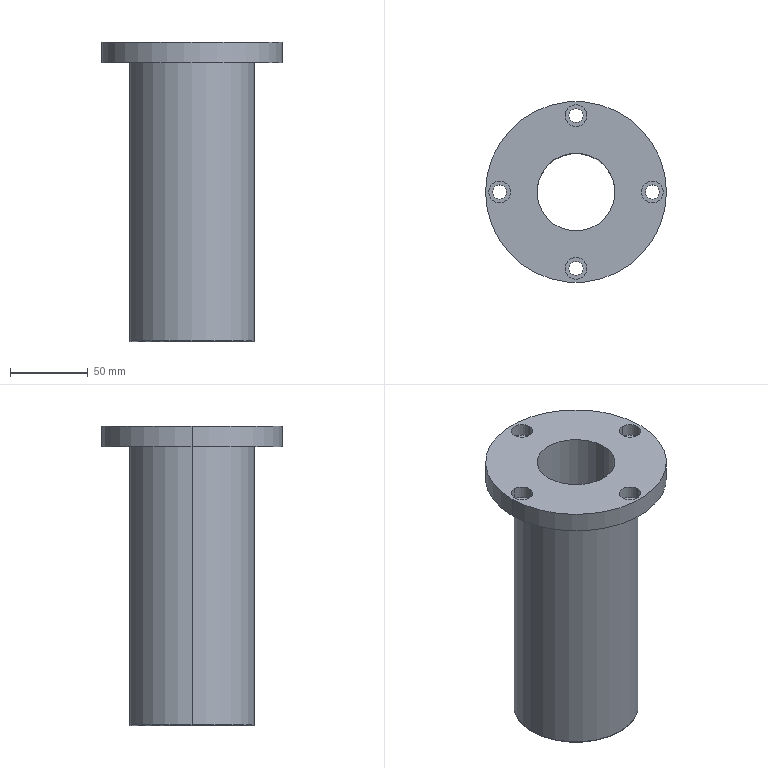Part | SolidWorks | features CirPattern 1, Fillet 1, ICE 1, RevCut 1, Revolution 1 | 1 solid | 31 faces | box 116 x 116 x 192 mm | volume 653901 mm3 | cylinder 22 | plane 7 | torus 2 | commonest cylinder face diameters 9 x8 14 x8 50 x2 80 x2 116 x2
STEP:
#1=CARTESIAN_POINT('',(49.,4.5,0.));
#2=VERTEX_POINT('',#1);
#3=CARTESIAN_POINT('',(49.,-4.5,0.));
#4=VERTEX_POINT('',#3);
#5=CARTESIAN_POINT('',(49.,0.,0.));
#6=DIRECTION('',(0.,0.,1.));
#7=DIRECTION('',(0.,-1.,0.));
#8=AXIS2_PLACEMENT_3D('',#5,#6,#7);
#9=CIRCLE('',#8,4.5);
#10=EDGE_CURVE('',#2,#4,#9,.T.);
#11=ORIENTED_EDGE('',*,*,#10,.F.);
#12=CARTESIAN_POINT('',(49.,4.5,4.9));
#13=VERTEX_POINT('',#12);
#14=CARTESIAN_POINT('',(49.,4.5,0.));
#15=DIRECTION('',(0.,0.,1.));
#16=VECTOR('',#15,1000.);
#17=LINE('',#14,#16);
#18=EDGE_CURVE('',#2,#13,#17,.T.);
#19=ORIENTED_EDGE('',*,*,#18,.T.);
#20=CARTESIAN_POINT('',(49.,-4.5,4.9));
#21=VERTEX_POINT('',#20);
#22=CARTESIAN_POINT('',(49.,0.,4.9));
#23=DIRECTION('',(0.,0.,1.));
#24=DIRECTION('',(0.,-1.,0.));
#25=AXIS2_PLACEMENT_3D('',#22,#23,#24);
#26=CIRCLE('',#25,4.5);
#27=EDGE_CURVE('',#13,#21,#26,.T.);
#28=ORIENTED_EDGE('',*,*,#27,.T.);
#29=CARTESIAN_POINT('',(49.,-4.5,0.));
#30=DIRECTION('',(0.,0.,1.));
#31=VECTOR('',#30,1000.);
#32=LINE('',#29,#31);
#33=EDGE_CURVE('',#4,#21,#32,.T.);
#34=ORIENTED_EDGE('',*,*,#33,.F.);
#35=EDGE_LOOP('',(#11,#19,#28,#34));
#36=FACE_OUTER_BOUND('',#35,.T.);
#37=CARTESIAN_POINT('',(49.,0.,0.));
#38=DIRECTION('',(0.,0.,1.));
#39=DIRECTION('',(0.,-1.,0.));
#40=AXIS2_PLACEMENT_3D('',#37,#38,#39);
#41=CYLINDRICAL_SURFACE('',#40,4.5);
#42=ADVANCED_FACE('',(#36),#41,.F.);
#43=CARTESIAN_POINT('',(49.,7.,4.9));
#44=VERTEX_POINT('',#43);
#45=CARTESIAN_POINT('',(49.,-7.,4.9));
#46=VERTEX_POINT('',#45);
#47=CARTESIAN_POINT('',(49.,0.,4.9));
#48=DIRECTION('',(0.,0.,1.));
#49=DIRECTION('',(0.,-1.,0.));
#50=AXIS2_PLACEMENT_3D('',#47,#48,#49);
#51=CIRCLE('',#50,7.);
#52=EDGE_CURVE('',#44,#46,#51,.T.);
#53=ORIENTED_EDGE('',*,*,#52,.F.);
#54=CARTESIAN_POINT('',(49.,7.,13.));
#55=VERTEX_POINT('',#54);
#56=CARTESIAN_POINT('',(49.,7.,0.));
#57=DIRECTION('',(0.,0.,1.));
#58=VECTOR('',#57,1000.);
#59=LINE('',#56,#58);
#60=EDGE_CURVE('',#44,#55,#59,.T.);
#61=ORIENTED_EDGE('',*,*,#60,.T.);
#62=CARTESIAN_POINT('',(49.,-7.,13.));
#63=VERTEX_POINT('',#62);
#64=CARTESIAN_POINT('',(49.,0.,13.));
#65=DIRECTION('',(0.,0.,1.));
#66=DIRECTION('',(0.,-1.,0.));
#67=AXIS2_PLACEMENT_3D('',#64,#65,#66);
#68=CIRCLE('',#67,7.);
#69=EDGE_CURVE('',#55,#63,#68,.T.);
#70=ORIENTED_EDGE('',*,*,#69,.T.);
#71=CARTESIAN_POINT('',(49.,-7.,0.));
#72=DIRECTION('',(0.,0.,1.));
#73=VECTOR('',#72,1000.);
#74=LINE('',#71,#73);
#75=EDGE_CURVE('',#46,#63,#74,.T.);
#76=ORIENTED_EDGE('',*,*,#75,.F.);
#77=EDGE_LOOP('',(#53,#61,#70,#76));
#78=FACE_OUTER_BOUND('',#77,.T.);
#79=CARTESIAN_POINT('',(49.,0.,0.));
#80=DIRECTION('',(0.,0.,1.));
#81=DIRECTION('',(0.,-1.,0.));
#82=AXIS2_PLACEMENT_3D('',#79,#80,#81);
#83=CYLINDRICAL_SURFACE('',#82,7.);
#84=ADVANCED_FACE('',(#78),#83,.F.);
#85=CARTESIAN_POINT('',(4.5,-49.,0.));
#86=VERTEX_POINT('',#85);
#87=CARTESIAN_POINT('',(-4.5,-49.,0.));
#88=VERTEX_POINT('',#87);
#89=CARTESIAN_POINT('',(0.,-49.,0.));
#90=DIRECTION('',(0.,0.,1.));
#91=DIRECTION('',(-1.,0.,0.));
#92=AXIS2_PLACEMENT_3D('',#89,#90,#91);
#93=CIRCLE('',#92,4.5);
#94=EDGE_CURVE('',#86,#88,#93,.T.);
#95=ORIENTED_EDGE('',*,*,#94,.F.);
#96=CARTESIAN_POINT('',(4.5,-49.,4.9));
#97=VERTEX_POINT('',#96);
#98=CARTESIAN_POINT('',(4.5,-49.,0.));
#99=DIRECTION('',(0.,0.,1.));
#100=VECTOR('',#99,1000.);
#101=LINE('',#98,#100);
#102=EDGE_CURVE('',#86,#97,#101,.T.);
#103=ORIENTED_EDGE('',*,*,#102,.T.);
#104=CARTESIAN_POINT('',(-4.5,-49.,4.9));
#105=VERTEX_POINT('',#104);
#106=CARTESIAN_POINT('',(0.,-49.,4.9));
#107=DIRECTION('',(0.,0.,1.));
#108=DIRECTION('',(-1.,0.,0.));
#109=AXIS2_PLACEMENT_3D('',#106,#107,#108);
#110=CIRCLE('',#109,4.5);
#111=EDGE_CURVE('',#97,#105,#110,.T.);
#112=ORIENTED_EDGE('',*,*,#111,.T.);
#113=CARTESIAN_POINT('',(-4.5,-49.,0.));
#114=DIRECTION('',(0.,0.,1.));
#115=VECTOR('',#114,1000.);
#116=LINE('',#113,#115);
#117=EDGE_CURVE('',#88,#105,#116,.T.);
#118=ORIENTED_EDGE('',*,*,#117,.F.);
#119=EDGE_LOOP('',(#95,#103,#112,#118));
#120=FACE_OUTER_BOUND('',#119,.T.);
#121=CARTESIAN_POINT('',(0.,-49.,0.));
#122=DIRECTION('',(0.,0.,1.));
#123=DIRECTION('',(-1.,0.,0.));
#124=AXIS2_PLACEMENT_3D('',#121,#122,#123);
#125=CYLINDRICAL_SURFACE('',#124,4.5);
#126=ADVANCED_FACE('',(#120),#125,.F.);
#127=CARTESIAN_POINT('',(7.,-49.,4.9));
#128=VERTEX_POINT('',#127);
#129=CARTESIAN_POINT('',(-7.,-49.,4.9));
#130=VERTEX_POINT('',#129);
#131=CARTESIAN_POINT('',(0.,-49.,4.9));
#132=DIRECTION('',(0.,0.,1.));
#133=DIRECTION('',(-1.,0.,0.));
#134=AXIS2_PLACEMENT_3D('',#131,#132,#133);
#135=CIRCLE('',#134,7.);
#136=EDGE_CURVE('',#128,#130,#135,.T.);
#137=ORIENTED_EDGE('',*,*,#136,.F.);
#138=CARTESIAN_POINT('',(7.,-49.,13.));
#139=VERTEX_POINT('',#138);
#140=CARTESIAN_POINT('',(7.,-49.,0.));
#141=DIRECTION('',(0.,0.,1.));
#142=VECTOR('',#141,1000.);
#143=LINE('',#140,#142);
#144=EDGE_CURVE('',#128,#139,#143,.T.);
#145=ORIENTED_EDGE('',*,*,#144,.T.);
#146=CARTESIAN_POINT('',(-7.,-49.,13.));
#147=VERTEX_POINT('',#146);
#148=CARTESIAN_POINT('',(0.,-49.,13.));
#149=DIRECTION('',(0.,0.,1.));
#150=DIRECTION('',(-1.,0.,0.));
#151=AXIS2_PLACEMENT_3D('',#148,#149,#150);
#152=CIRCLE('',#151,7.);
#153=EDGE_CURVE('',#139,#147,#152,.T.);
#154=ORIENTED_EDGE('',*,*,#153,.T.);
#155=CARTESIAN_POINT('',(-7.,-49.,0.));
#156=DIRECTION('',(0.,0.,1.));
#157=VECTOR('',#156,1000.);
#158=LINE('',#155,#157);
#159=EDGE_CURVE('',#130,#147,#158,.T.);
#160=ORIENTED_EDGE('',*,*,#159,.F.);
#161=EDGE_LOOP('',(#137,#145,#154,#160));
#162=FACE_OUTER_BOUND('',#161,.T.);
#163=CARTESIAN_POINT('',(0.,-49.,0.));
#164=DIRECTION('',(0.,0.,1.));
#165=DIRECTION('',(-1.,0.,0.));
#166=AXIS2_PLACEMENT_3D('',#163,#164,#165);
#167=CYLINDRICAL_SURFACE('',#166,7.);
#168=ADVANCED_FACE('',(#162),#167,.F.);
#169=CARTESIAN_POINT('',(-49.,-4.5,0.));
#170=VERTEX_POINT('',#169);
#171=CARTESIAN_POINT('',(-49.,4.5,0.));
#172=VERTEX_POINT('',#171);
#173=CARTESIAN_POINT('',(-49.,0.,0.));
#174=DIRECTION('',(0.,0.,1.));
#175=DIRECTION('',(0.,1.,0.));
#176=AXIS2_PLACEMENT_3D('',#173,#174,#175);
#177=CIRCLE('',#176,4.5);
#178=EDGE_CURVE('',#170,#172,#177,.T.);
#179=ORIENTED_EDGE('',*,*,#178,.F.);
#180=CARTESIAN_POINT('',(-49.,-4.5,4.9));
#181=VERTEX_POINT('',#180);
#182=CARTESIAN_POINT('',(-49.,-4.5,0.));
#183=DIRECTION('',(0.,0.,1.));
#184=VECTOR('',#183,1000.);
#185=LINE('',#182,#184);
#186=EDGE_CURVE('',#170,#181,#185,.T.);
#187=ORIENTED_EDGE('',*,*,#186,.T.);
#188=CARTESIAN_POINT('',(-49.,4.5,4.9));
#189=VERTEX_POINT('',#188);
#190=CARTESIAN_POINT('',(-49.,0.,4.9));
#191=DIRECTION('',(0.,0.,1.));
#192=DIRECTION('',(0.,1.,0.));
#193=AXIS2_PLACEMENT_3D('',#190,#191,#192);
#194=CIRCLE('',#193,4.5);
#195=EDGE_CURVE('',#181,#189,#194,.T.);
#196=ORIENTED_EDGE('',*,*,#195,.T.);
#197=CARTESIAN_POINT('',(-49.,4.5,0.));
#198=DIRECTION('',(0.,0.,1.));
#199=VECTOR('',#198,1000.);
#200=LINE('',#197,#199);
#201=EDGE_CURVE('',#172,#189,#200,.T.);
#202=ORIENTED_EDGE('',*,*,#201,.F.);
#203=EDGE_LOOP('',(#179,#187,#196,#202));
#204=FACE_OUTER_BOUND('',#203,.T.);
#205=CARTESIAN_POINT('',(-49.,0.,0.));
#206=DIRECTION('',(0.,0.,1.));
#207=DIRECTION('',(0.,1.,0.));
#208=AXIS2_PLACEMENT_3D('',#205,#206,#207);
#209=CYLINDRICAL_SURFACE('',#208,4.5);
#210=ADVANCED_FACE('',(#204),#209,.F.);
#211=CARTESIAN_POINT('',(-49.,-7.,4.9));
#212=VERTEX_POINT('',#211);
#213=CARTESIAN_POINT('',(-49.,7.,4.9));
#214=VERTEX_POINT('',#213);
#215=CARTESIAN_POINT('',(-49.,0.,4.9));
#216=DIRECTION('',(0.,0.,1.));
#217=DIRECTION('',(0.,1.,0.));
#218=AXIS2_PLACEMENT_3D('',#215,#216,#217);
#219=CIRCLE('',#218,7.);
#220=EDGE_CURVE('',#212,#214,#219,.T.);
#221=ORIENTED_EDGE('',*,*,#220,.F.);
#222=CARTESIAN_POINT('',(-49.,-7.,13.));
#223=VERTEX_POINT('',#222);
#224=CARTESIAN_POINT('',(-49.,-7.,0.));
#225=DIRECTION('',(0.,0.,1.));
#226=VECTOR('',#225,1000.);
#227=LINE('',#224,#226);
#228=EDGE_CURVE('',#212,#223,#227,.T.);
#229=ORIENTED_EDGE('',*,*,#228,.T.);
#230=CARTESIAN_POINT('',(-49.,7.,13.));
#231=VERTEX_POINT('',#230);
#232=CARTESIAN_POINT('',(-49.,0.,13.));
#233=DIRECTION('',(0.,0.,1.));
#234=DIRECTION('',(0.,1.,0.));
#235=AXIS2_PLACEMENT_3D('',#232,#233,#234);
#236=CIRCLE('',#235,7.);
#237=EDGE_CURVE('',#223,#231,#236,.T.);
#238=ORIENTED_EDGE('',*,*,#237,.T.);
#239=CARTESIAN_POINT('',(-49.,7.,0.));
#240=DIRECTION('',(0.,0.,1.));
#241=VECTOR('',#240,1000.);
#242=LINE('',#239,#241);
#243=EDGE_CURVE('',#214,#231,#242,.T.);
#244=ORIENTED_EDGE('',*,*,#243,.F.);
#245=EDGE_LOOP('',(#221,#229,#238,#244));
#246=FACE_OUTER_BOUND('',#245,.T.);
#247=CARTESIAN_POINT('',(-49.,0.,0.));
#248=DIRECTION('',(0.,0.,1.));
#249=DIRECTION('',(0.,1.,0.));
#250=AXIS2_PLACEMENT_3D('',#247,#248,#249);
#251=CYLINDRICAL_SURFACE('',#250,7.);
#252=ADVANCED_FACE('',(#246),#251,.F.);
#253=CARTESIAN_POINT('',(-4.5,49.,0.));
#254=VERTEX_POINT('',#253);
#255=CARTESIAN_POINT('',(4.5,49.,0.));
#256=VERTEX_POINT('',#255);
#257=CARTESIAN_POINT('',(0.,49.,0.));
#258=DIRECTION('',(0.,0.,1.));
#259=DIRECTION('',(1.,0.,0.));
#260=AXIS2_PLACEMENT_3D('',#257,#258,#259);
#261=CIRCLE('',#260,4.5);
#262=EDGE_CURVE('',#254,#256,#261,.T.);
#263=ORIENTED_EDGE('',*,*,#262,.F.);
#264=CARTESIAN_POINT('',(-4.5,49.,4.9));
#265=VERTEX_POINT('',#264);
#266=CARTESIAN_POINT('',(-4.5,49.,0.));
#267=DIRECTION('',(0.,0.,1.));
#268=VECTOR('',#267,1000.);
#269=LINE('',#266,#268);
#270=EDGE_CURVE('',#254,#265,#269,.T.);
#271=ORIENTED_EDGE('',*,*,#270,.T.);
#272=CARTESIAN_POINT('',(4.5,49.,4.9));
#273=VERTEX_POINT('',#272);
#274=CARTESIAN_POINT('',(0.,49.,4.9));
#275=DIRECTION('',(0.,0.,1.));
#276=DIRECTION('',(1.,0.,0.));
#277=AXIS2_PLACEMENT_3D('',#274,#275,#276);
#278=CIRCLE('',#277,4.5);
#279=EDGE_CURVE('',#265,#273,#278,.T.);
#280=ORIENTED_EDGE('',*,*,#279,.T.);
#281=CARTESIAN_POINT('',(4.5,49.,0.));
#282=DIRECTION('',(0.,0.,1.));
#283=VECTOR('',#282,1000.);
#284=LINE('',#281,#283);
#285=EDGE_CURVE('',#256,#273,#284,.T.);
#286=ORIENTED_EDGE('',*,*,#285,.F.);
#287=EDGE_LOOP('',(#263,#271,#280,#286));
#288=FACE_OUTER_BOUND('',#287,.T.);
#289=CARTESIAN_POINT('',(0.,49.,0.));
#290=DIRECTION('',(0.,0.,1.));
#291=DIRECTION('',(1.,0.,0.));
#292=AXIS2_PLACEMENT_3D('',#289,#290,#291);
#293=CYLINDRICAL_SURFACE('',#292,4.5);
#294=ADVANCED_FACE('',(#288),#293,.F.);
#295=CARTESIAN_POINT('',(-7.,49.,4.9));
#296=VERTEX_POINT('',#295);
#297=CARTESIAN_POINT('',(7.,49.,4.9));
#298=VERTEX_POINT('',#297);
#299=CARTESIAN_POINT('',(0.,49.,4.9));
#300=DIRECTION('',(0.,0.,1.));
#301=DIRECTION('',(1.,0.,0.));
#302=AXIS2_PLACEMENT_3D('',#299,#300,#301);
#303=CIRCLE('',#302,7.);
#304=EDGE_CURVE('',#296,#298,#303,.T.);
#305=ORIENTED_EDGE('',*,*,#304,.F.);
#306=CARTESIAN_POINT('',(-7.,49.,13.));
#307=VERTEX_POINT('',#306);
#308=CARTESIAN_POINT('',(-7.,49.,0.));
#309=DIRECTION('',(0.,0.,1.));
#310=VECTOR('',#309,1000.);
#311=LINE('',#308,#310);
#312=EDGE_CURVE('',#296,#307,#311,.T.);
#313=ORIENTED_EDGE('',*,*,#312,.T.);
#314=CARTESIAN_POINT('',(7.,49.,13.));
#315=VERTEX_POINT('',#314);
#316=CARTESIAN_POINT('',(0.,49.,13.));
#317=DIRECTION('',(0.,0.,1.));
#318=DIRECTION('',(1.,0.,0.));
#319=AXIS2_PLACEMENT_3D('',#316,#317,#318);
#320=CIRCLE('',#319,7.);
#321=EDGE_CURVE('',#307,#315,#320,.T.);
#322=ORIENTED_EDGE('',*,*,#321,.T.);
#323=CARTESIAN_POINT('',(7.,49.,0.));
#324=DIRECTION('',(0.,0.,1.));
#325=VECTOR('',#324,1000.);
#326=LINE('',#323,#325);
#327=EDGE_CURVE('',#298,#315,#326,.T.);
#328=ORIENTED_EDGE('',*,*,#327,.F.);
#329=EDGE_LOOP('',(#305,#313,#322,#328));
#330=FACE_OUTER_BOUND('',#329,.T.);
#331=CARTESIAN_POINT('',(0.,49.,0.));
#332=DIRECTION('',(0.,0.,1.));
#333=DIRECTION('',(1.,0.,0.));
#334=AXIS2_PLACEMENT_3D('',#331,#332,#333);
#335=CYLINDRICAL_SURFACE('',#334,7.);
#336=ADVANCED_FACE('',(#330),#335,.F.);
#337=CARTESIAN_POINT('',(58.,0.,13.));
#338=VERTEX_POINT('',#337);
#339=CARTESIAN_POINT('',(-58.,0.,13.));
#340=VERTEX_POINT('',#339);
#341=CARTESIAN_POINT('',(0.,0.,13.));
#342=DIRECTION('',(0.,0.,1.));
#343=DIRECTION('',(1.,0.,0.));
#344=AXIS2_PLACEMENT_3D('',#341,#342,#343);
#345=CIRCLE('',#344,58.);
#346=EDGE_CURVE('',#338,#340,#345,.T.);
#347=ORIENTED_EDGE('',*,*,#346,.F.);
#348=CARTESIAN_POINT('',(58.,0.,0.));
#349=VERTEX_POINT('',#348);
#350=CARTESIAN_POINT('',(58.,0.,13.));
#351=DIRECTION('',(0.,0.,-1.));
#352=VECTOR('',#351,1000.);
#353=LINE('',#350,#352);
#354=EDGE_CURVE('',#338,#349,#353,.T.);
#355=ORIENTED_EDGE('',*,*,#354,.T.);
#356=CARTESIAN_POINT('',(-58.,0.,0.));
#357=VERTEX_POINT('',#356);
#358=CARTESIAN_POINT('',(0.,0.,0.));
#359=DIRECTION('',(0.,0.,1.));
#360=DIRECTION('',(1.,0.,0.));
#361=AXIS2_PLACEMENT_3D('',#358,#359,#360);
#362=CIRCLE('',#361,58.);
#363=EDGE_CURVE('',#349,#357,#362,.T.);
#364=ORIENTED_EDGE('',*,*,#363,.T.);
#365=CARTESIAN_POINT('',(-58.,0.,13.));
#366=DIRECTION('',(0.,0.,-1.));
#367=VECTOR('',#366,1000.);
#368=LINE('',#365,#367);
#369=EDGE_CURVE('',#340,#357,#368,.T.);
#370=ORIENTED_EDGE('',*,*,#369,.F.);
#371=EDGE_LOOP('',(#347,#355,#364,#370));
#372=FACE_OUTER_BOUND('',#371,.T.);
#373=CARTESIAN_POINT('',(0.,0.,13.));
#374=DIRECTION('',(0.,0.,-1.));
#375=DIRECTION('',(-1.,0.,0.));
#376=AXIS2_PLACEMENT_3D('',#373,#374,#375);
#377=CYLINDRICAL_SURFACE('',#376,58.);
#378=ADVANCED_FACE('',(#372),#377,.T.);
#379=CARTESIAN_POINT('',(-39.5,0.,-179.));
#380=VERTEX_POINT('',#379);
#381=CARTESIAN_POINT('',(39.5,0.,-179.));
#382=VERTEX_POINT('',#381);
#383=CARTESIAN_POINT('',(0.,0.,-179.));
#384=DIRECTION('',(0.,0.,-1.));
#385=DIRECTION('',(1.,0.,0.));
#386=AXIS2_PLACEMENT_3D('',#383,#384,#385);
#387=CIRCLE('',#386,39.5);
#388=EDGE_CURVE('',#380,#382,#387,.T.);
#389=ORIENTED_EDGE('',*,*,#388,.F.);
#390=CARTESIAN_POINT('',(-40.,0.,-178.5));
#391=VERTEX_POINT('',#390);
#392=CARTESIAN_POINT('',(-39.5,0.,-178.5));
#393=DIRECTION('',(0.,1.,0.));
#394=DIRECTION('',(-1.,0.,0.));
#395=AXIS2_PLACEMENT_3D('',#392,#393,#394);
#396=CIRCLE('',#395,0.5);
#397=EDGE_CURVE('',#380,#391,#396,.T.);
#398=ORIENTED_EDGE('',*,*,#397,.T.);
#399=CARTESIAN_POINT('',(40.,0.,-178.5));
#400=VERTEX_POINT('',#399);
#401=CARTESIAN_POINT('',(0.,0.,-178.5));
#402=DIRECTION('',(0.,0.,1.));
#403=DIRECTION('',(1.,0.,0.));
#404=AXIS2_PLACEMENT_3D('',#401,#402,#403);
#405=CIRCLE('',#404,40.);
#406=EDGE_CURVE('',#400,#391,#405,.T.);
#407=ORIENTED_EDGE('',*,*,#406,.F.);
#408=CARTESIAN_POINT('',(39.5,0.,-178.5));
#409=DIRECTION('',(0.,-1.,0.));
#410=DIRECTION('',(0.,0.,-1.));
#411=AXIS2_PLACEMENT_3D('',#408,#409,#410);
#412=CIRCLE('',#411,0.5);
#413=EDGE_CURVE('',#382,#400,#412,.T.);
#414=ORIENTED_EDGE('',*,*,#413,.F.);
#415=EDGE_LOOP('',(#389,#398,#407,#414));
#416=FACE_OUTER_BOUND('',#415,.T.);
#417=CARTESIAN_POINT('',(0.,0.,-178.5));
#418=DIRECTION('',(0.,0.,1.));
#419=DIRECTION('',(1.,0.,0.));
#420=AXIS2_PLACEMENT_3D('',#417,#418,#419);
#421=TOROIDAL_SURFACE('',#420,39.5,0.5);
#422=ADVANCED_FACE('',(#416),#421,.T.);
#423=ORIENTED_EDGE('',*,*,#406,.T.);
#424=CARTESIAN_POINT('',(-40.,0.,0.));
#425=VERTEX_POINT('',#424);
#426=CARTESIAN_POINT('',(-40.,0.,0.));
#427=DIRECTION('',(0.,0.,1.));
#428=VECTOR('',#427,1000.);
#429=LINE('',#426,#428);
#430=EDGE_CURVE('',#391,#425,#429,.T.);
#431=ORIENTED_EDGE('',*,*,#430,.T.);
#432=CARTESIAN_POINT('',(40.,0.,0.));
#433=VERTEX_POINT('',#432);
#434=CARTESIAN_POINT('',(0.,0.,0.));
#435=DIRECTION('',(0.,0.,1.));
#436=DIRECTION('',(1.,0.,0.));
#437=AXIS2_PLACEMENT_3D('',#434,#435,#436);
#438=CIRCLE('',#437,40.);
#439=EDGE_CURVE('',#433,#425,#438,.T.);
#440=ORIENTED_EDGE('',*,*,#439,.F.);
#441=CARTESIAN_POINT('',(40.,0.,0.));
#442=DIRECTION('',(0.,0.,1.));
#443=VECTOR('',#442,1000.);
#444=LINE('',#441,#443);
#445=EDGE_CURVE('',#400,#433,#444,.T.);
#446=ORIENTED_EDGE('',*,*,#445,.F.);
#447=EDGE_LOOP('',(#423,#431,#440,#446));
#448=FACE_OUTER_BOUND('',#447,.T.);
#449=CARTESIAN_POINT('',(0.,0.,0.));
#450=DIRECTION('',(0.,0.,1.));
#451=DIRECTION('',(1.,0.,0.));
#452=AXIS2_PLACEMENT_3D('',#449,#450,#451);
#453=CYLINDRICAL_SURFACE('',#452,40.);
#454=ADVANCED_FACE('',(#448),#453,.T.);
#455=CARTESIAN_POINT('',(-25.,0.,-179.));
#456=VERTEX_POINT('',#455);
#457=CARTESIAN_POINT('',(25.,0.,-179.));
#458=VERTEX_POINT('',#457);
#459=CARTESIAN_POINT('',(0.,0.,-179.));
#460=DIRECTION('',(0.,0.,1.));
#461=DIRECTION('',(1.,0.,0.));
#462=AXIS2_PLACEMENT_3D('',#459,#460,#461);
#463=CIRCLE('',#462,25.);
#464=EDGE_CURVE('',#456,#458,#463,.T.);
#465=ORIENTED_EDGE('',*,*,#464,.F.);
#466=CARTESIAN_POINT('',(-25.,0.,13.));
#467=VERTEX_POINT('',#466);
#468=CARTESIAN_POINT('',(-25.,0.,0.));
#469=DIRECTION('',(0.,0.,1.));
#470=VECTOR('',#469,1000.);
#471=LINE('',#468,#470);
#472=EDGE_CURVE('',#456,#467,#471,.T.);
#473=ORIENTED_EDGE('',*,*,#472,.T.);
#474=CARTESIAN_POINT('',(25.,0.,13.));
#475=VERTEX_POINT('',#474);
#476=CARTESIAN_POINT('',(0.,0.,13.));
#477=DIRECTION('',(0.,0.,1.));
#478=DIRECTION('',(1.,0.,0.));
#479=AXIS2_PLACEMENT_3D('',#476,#477,#478);
#480=CIRCLE('',#479,25.);
#481=EDGE_CURVE('',#467,#475,#480,.T.);
#482=ORIENTED_EDGE('',*,*,#481,.T.);
#483=CARTESIAN_POINT('',(25.,0.,0.));
#484=DIRECTION('',(0.,0.,1.));
#485=VECTOR('',#484,1000.);
#486=LINE('',#483,#485);
#487=EDGE_CURVE('',#458,#475,#486,.T.);
#488=ORIENTED_EDGE('',*,*,#487,.F.);
#489=EDGE_LOOP('',(#465,#473,#482,#488));
#490=FACE_OUTER_BOUND('',#489,.T.);
#491=CARTESIAN_POINT('',(0.,0.,0.));
#492=DIRECTION('',(0.,0.,1.));
#493=DIRECTION('',(1.,0.,0.));
#494=AXIS2_PLACEMENT_3D('',#491,#492,#493);
#495=CYLINDRICAL_SURFACE('',#494,25.);
#496=ADVANCED_FACE('',(#490),#495,.F.);
#497=ORIENTED_EDGE('',*,*,#472,.F.);
#498=CARTESIAN_POINT('',(0.,0.,-179.));
#499=DIRECTION('',(0.,0.,1.));
#500=DIRECTION('',(1.,0.,0.));
#501=AXIS2_PLACEMENT_3D('',#498,#499,#500);
#502=CIRCLE('',#501,25.);
#503=EDGE_CURVE('',#458,#456,#502,.T.);
#504=ORIENTED_EDGE('',*,*,#503,.F.);
#505=ORIENTED_EDGE('',*,*,#487,.T.);
#506=CARTESIAN_POINT('',(0.,0.,13.));
#507=DIRECTION('',(0.,0.,1.));
#508=DIRECTION('',(1.,0.,0.));
#509=AXIS2_PLACEMENT_3D('',#506,#507,#508);
#510=CIRCLE('',#509,25.);
#511=EDGE_CURVE('',#475,#467,#510,.T.);
#512=ORIENTED_EDGE('',*,*,#511,.T.);
#513=EDGE_LOOP('',(#497,#504,#505,#512));
#514=FACE_OUTER_BOUND('',#513,.T.);
#515=CARTESIAN_POINT('',(0.,0.,0.));
#516=DIRECTION('',(0.,0.,1.));
#517=DIRECTION('',(1.,0.,0.));
#518=AXIS2_PLACEMENT_3D('',#515,#516,#517);
#519=CYLINDRICAL_SURFACE('',#518,25.);
#520=ADVANCED_FACE('',(#514),#519,.F.);
#521=CARTESIAN_POINT('',(0.,0.,-179.));
#522=DIRECTION('',(0.,0.,-1.));
#523=DIRECTION('',(1.,0.,0.));
#524=AXIS2_PLACEMENT_3D('',#521,#522,#523);
#525=CIRCLE('',#524,39.5);
#526=EDGE_CURVE('',#382,#380,#525,.T.);
#527=ORIENTED_EDGE('',*,*,#526,.T.);
#528=ORIENTED_EDGE('',*,*,#388,.T.);
#529=EDGE_LOOP('',(#527,#528));
#530=FACE_OUTER_BOUND('',#529,.T.);
#531=ORIENTED_EDGE('',*,*,#503,.T.);
#532=ORIENTED_EDGE('',*,*,#464,.T.);
#533=EDGE_LOOP('',(#531,#532));
#534=FACE_BOUND('',#533,.T.);
#535=CARTESIAN_POINT('',(0.,40.,-179.));
#536=DIRECTION('',(0.,0.,1.));
#537=DIRECTION('',(1.,0.,0.));
#538=AXIS2_PLACEMENT_3D('',#535,#536,#537);
#539=PLANE('',#538);
#540=ADVANCED_FACE('',(#530,#534),#539,.F.);
#541=ORIENTED_EDGE('',*,*,#430,.F.);
#542=CARTESIAN_POINT('',(0.,0.,-178.5));
#543=DIRECTION('',(0.,0.,1.));
#544=DIRECTION('',(1.,0.,0.));
#545=AXIS2_PLACEMENT_3D('',#542,#543,#544);
#546=CIRCLE('',#545,40.);
#547=EDGE_CURVE('',#391,#400,#546,.T.);
#548=ORIENTED_EDGE('',*,*,#547,.T.);
#549=ORIENTED_EDGE('',*,*,#445,.T.);
#550=CARTESIAN_POINT('',(0.,0.,0.));
#551=DIRECTION('',(0.,0.,1.));
#552=DIRECTION('',(1.,0.,0.));
#553=AXIS2_PLACEMENT_3D('',#550,#551,#552);
#554=CIRCLE('',#553,40.);
#555=EDGE_CURVE('',#425,#433,#554,.T.);
#556=ORIENTED_EDGE('',*,*,#555,.F.);
#557=EDGE_LOOP('',(#541,#548,#549,#556));
#558=FACE_OUTER_BOUND('',#557,.T.);
#559=CARTESIAN_POINT('',(0.,0.,0.));
#560=DIRECTION('',(0.,0.,1.));
#561=DIRECTION('',(1.,0.,0.));
#562=AXIS2_PLACEMENT_3D('',#559,#560,#561);
#563=CYLINDRICAL_SURFACE('',#562,40.);
#564=ADVANCED_FACE('',(#558),#563,.T.);
#565=ORIENTED_EDGE('',*,*,#397,.F.);
#566=ORIENTED_EDGE('',*,*,#526,.F.);
#567=ORIENTED_EDGE('',*,*,#413,.T.);
#568=ORIENTED_EDGE('',*,*,#547,.F.);
#569=EDGE_LOOP('',(#565,#566,#567,#568));
#570=FACE_OUTER_BOUND('',#569,.T.);
#571=CARTESIAN_POINT('',(0.,0.,-178.5));
#572=DIRECTION('',(0.,0.,1.));
#573=DIRECTION('',(1.,0.,0.));
#574=AXIS2_PLACEMENT_3D('',#571,#572,#573);
#575=TOROIDAL_SURFACE('',#574,39.5,0.5);
#576=ADVANCED_FACE('',(#570),#575,.T.);
#577=CARTESIAN_POINT('',(49.,0.,0.));
#578=DIRECTION('',(0.,0.,1.));
#579=DIRECTION('',(0.,-1.,0.));
#580=AXIS2_PLACEMENT_3D('',#577,#578,#579);
#581=CIRCLE('',#580,4.5);
#582=EDGE_CURVE('',#4,#2,#581,.T.);
#583=ORIENTED_EDGE('',*,*,#582,.T.);
#584=ORIENTED_EDGE('',*,*,#10,.T.);
#585=EDGE_LOOP('',(#583,#584));
#586=FACE_BOUND('',#585,.T.);
#587=CARTESIAN_POINT('',(0.,-49.,0.));
#588=DIRECTION('',(0.,0.,1.));
#589=DIRECTION('',(-1.,0.,0.));
#590=AXIS2_PLACEMENT_3D('',#587,#588,#589);
#591=CIRCLE('',#590,4.5);
#592=EDGE_CURVE('',#88,#86,#591,.T.);
#593=ORIENTED_EDGE('',*,*,#592,.T.);
#594=ORIENTED_EDGE('',*,*,#94,.T.);
#595=EDGE_LOOP('',(#593,#594));
#596=FACE_BOUND('',#595,.T.);
#597=CARTESIAN_POINT('',(-49.,0.,0.));
#598=DIRECTION('',(0.,0.,1.));
#599=DIRECTION('',(0.,1.,0.));
#600=AXIS2_PLACEMENT_3D('',#597,#598,#599);
#601=CIRCLE('',#600,4.5);
#602=EDGE_CURVE('',#172,#170,#601,.T.);
#603=ORIENTED_EDGE('',*,*,#602,.T.);
#604=ORIENTED_EDGE('',*,*,#178,.T.);
#605=EDGE_LOOP('',(#603,#604));
#606=FACE_BOUND('',#605,.T.);
#607=CARTESIAN_POINT('',(0.,49.,0.));
#608=DIRECTION('',(0.,0.,1.));
#609=DIRECTION('',(1.,0.,0.));
#610=AXIS2_PLACEMENT_3D('',#607,#608,#609);
#611=CIRCLE('',#610,4.5);
#612=EDGE_CURVE('',#256,#254,#611,.T.);
#613=ORIENTED_EDGE('',*,*,#612,.T.);
#614=ORIENTED_EDGE('',*,*,#262,.T.);
#615=EDGE_LOOP('',(#613,#614));
#616=FACE_BOUND('',#615,.T.);
#617=CARTESIAN_POINT('',(0.,0.,0.));
#618=DIRECTION('',(0.,0.,1.));
#619=DIRECTION('',(1.,0.,0.));
#620=AXIS2_PLACEMENT_3D('',#617,#618,#619);
#621=CIRCLE('',#620,58.);
#622=EDGE_CURVE('',#357,#349,#621,.T.);
#623=ORIENTED_EDGE('',*,*,#622,.F.);
#624=ORIENTED_EDGE('',*,*,#363,.F.);
#625=EDGE_LOOP('',(#623,#624));
#626=FACE_OUTER_BOUND('',#625,.T.);
#627=ORIENTED_EDGE('',*,*,#439,.T.);
#628=ORIENTED_EDGE('',*,*,#555,.T.);
#629=EDGE_LOOP('',(#627,#628));
#630=FACE_BOUND('',#629,.T.);
#631=CARTESIAN_POINT('',(0.,0.,0.));
#632=DIRECTION('',(0.,0.,1.));
#633=DIRECTION('',(1.,0.,0.));
#634=AXIS2_PLACEMENT_3D('',#631,#632,#633);
#635=PLANE('',#634);
#636=ADVANCED_FACE('',(#586,#596,#606,#616,#626,#630),#635,.F.);
#637=CARTESIAN_POINT('',(49.,0.,13.));
#638=DIRECTION('',(0.,0.,1.));
#639=DIRECTION('',(0.,-1.,0.));
#640=AXIS2_PLACEMENT_3D('',#637,#638,#639);
#641=CIRCLE('',#640,7.);
#642=EDGE_CURVE('',#63,#55,#641,.T.);
#643=ORIENTED_EDGE('',*,*,#642,.F.);
#644=ORIENTED_EDGE('',*,*,#69,.F.);
#645=EDGE_LOOP('',(#643,#644));
#646=FACE_BOUND('',#645,.T.);
#647=CARTESIAN_POINT('',(0.,-49.,13.));
#648=DIRECTION('',(0.,0.,1.));
#649=DIRECTION('',(-1.,0.,0.));
#650=AXIS2_PLACEMENT_3D('',#647,#648,#649);
#651=CIRCLE('',#650,7.);
#652=EDGE_CURVE('',#147,#139,#651,.T.);
#653=ORIENTED_EDGE('',*,*,#652,.F.);
#654=ORIENTED_EDGE('',*,*,#153,.F.);
#655=EDGE_LOOP('',(#653,#654));
#656=FACE_BOUND('',#655,.T.);
#657=CARTESIAN_POINT('',(-49.,0.,13.));
#658=DIRECTION('',(0.,0.,1.));
#659=DIRECTION('',(0.,1.,0.));
#660=AXIS2_PLACEMENT_3D('',#657,#658,#659);
#661=CIRCLE('',#660,7.);
#662=EDGE_CURVE('',#231,#223,#661,.T.);
#663=ORIENTED_EDGE('',*,*,#662,.F.);
#664=ORIENTED_EDGE('',*,*,#237,.F.);
#665=EDGE_LOOP('',(#663,#664));
#666=FACE_BOUND('',#665,.T.);
#667=CARTESIAN_POINT('',(0.,49.,13.));
#668=DIRECTION('',(0.,0.,1.));
#669=DIRECTION('',(1.,0.,0.));
#670=AXIS2_PLACEMENT_3D('',#667,#668,#669);
#671=CIRCLE('',#670,7.);
#672=EDGE_CURVE('',#315,#307,#671,.T.);
#673=ORIENTED_EDGE('',*,*,#672,.F.);
#674=ORIENTED_EDGE('',*,*,#321,.F.);
#675=EDGE_LOOP('',(#673,#674));
#676=FACE_BOUND('',#675,.T.);
#677=CARTESIAN_POINT('',(0.,0.,13.));
#678=DIRECTION('',(0.,0.,1.));
#679=DIRECTION('',(1.,0.,0.));
#680=AXIS2_PLACEMENT_3D('',#677,#678,#679);
#681=CIRCLE('',#680,58.);
#682=EDGE_CURVE('',#340,#338,#681,.T.);
#683=ORIENTED_EDGE('',*,*,#682,.T.);
#684=ORIENTED_EDGE('',*,*,#346,.T.);
#685=EDGE_LOOP('',(#683,#684));
#686=FACE_OUTER_BOUND('',#685,.T.);
#687=ORIENTED_EDGE('',*,*,#511,.F.);
#688=ORIENTED_EDGE('',*,*,#481,.F.);
#689=EDGE_LOOP('',(#687,#688));
#690=FACE_BOUND('',#689,.T.);
#691=CARTESIAN_POINT('',(0.,0.,13.));
#692=DIRECTION('',(0.,0.,1.));
#693=DIRECTION('',(1.,0.,0.));
#694=AXIS2_PLACEMENT_3D('',#691,#692,#693);
#695=PLANE('',#694);
#696=ADVANCED_FACE('',(#646,#656,#666,#676,#686,#690),#695,.T.);
#697=ORIENTED_EDGE('',*,*,#354,.F.);
#698=ORIENTED_EDGE('',*,*,#682,.F.);
#699=ORIENTED_EDGE('',*,*,#369,.T.);
#700=ORIENTED_EDGE('',*,*,#622,.T.);
#701=EDGE_LOOP('',(#697,#698,#699,#700));
#702=FACE_OUTER_BOUND('',#701,.T.);
#703=CARTESIAN_POINT('',(0.,0.,13.));
#704=DIRECTION('',(0.,0.,-1.));
#705=DIRECTION('',(-1.,0.,0.));
#706=AXIS2_PLACEMENT_3D('',#703,#704,#705);
#707=CYLINDRICAL_SURFACE('',#706,58.);
#708=ADVANCED_FACE('',(#702),#707,.T.);
#709=CARTESIAN_POINT('',(0.,49.,4.9));
#710=DIRECTION('',(0.,0.,1.));
#711=DIRECTION('',(1.,0.,0.));
#712=AXIS2_PLACEMENT_3D('',#709,#710,#711);
#713=CIRCLE('',#712,4.5);
#714=EDGE_CURVE('',#273,#265,#713,.T.);
#715=ORIENTED_EDGE('',*,*,#714,.F.);
#716=ORIENTED_EDGE('',*,*,#279,.F.);
#717=EDGE_LOOP('',(#715,#716));
#718=FACE_BOUND('',#717,.T.);
#719=CARTESIAN_POINT('',(0.,49.,4.9));
#720=DIRECTION('',(0.,0.,1.));
#721=DIRECTION('',(1.,0.,0.));
#722=AXIS2_PLACEMENT_3D('',#719,#720,#721);
#723=CIRCLE('',#722,7.);
#724=EDGE_CURVE('',#298,#296,#723,.T.);
#725=ORIENTED_EDGE('',*,*,#724,.T.);
#726=ORIENTED_EDGE('',*,*,#304,.T.);
#727=EDGE_LOOP('',(#725,#726));
#728=FACE_OUTER_BOUND('',#727,.T.);
#729=CARTESIAN_POINT('',(0.,0.,4.9));
#730=DIRECTION('',(0.,0.,-1.));
#731=DIRECTION('',(-1.,0.,0.));
#732=AXIS2_PLACEMENT_3D('',#729,#730,#731);
#733=PLANE('',#732);
#734=ADVANCED_FACE('',(#718,#728),#733,.F.);
#735=ORIENTED_EDGE('',*,*,#312,.F.);
#736=ORIENTED_EDGE('',*,*,#724,.F.);
#737=ORIENTED_EDGE('',*,*,#327,.T.);
#738=ORIENTED_EDGE('',*,*,#672,.T.);
#739=EDGE_LOOP('',(#735,#736,#737,#738));
#740=FACE_OUTER_BOUND('',#739,.T.);
#741=CARTESIAN_POINT('',(0.,49.,0.));
#742=DIRECTION('',(0.,0.,1.));
#743=DIRECTION('',(1.,0.,0.));
#744=AXIS2_PLACEMENT_3D('',#741,#742,#743);
#745=CYLINDRICAL_SURFACE('',#744,7.);
#746=ADVANCED_FACE('',(#740),#745,.F.);
#747=ORIENTED_EDGE('',*,*,#270,.F.);
#748=ORIENTED_EDGE('',*,*,#612,.F.);
#749=ORIENTED_EDGE('',*,*,#285,.T.);
#750=ORIENTED_EDGE('',*,*,#714,.T.);
#751=EDGE_LOOP('',(#747,#748,#749,#750));
#752=FACE_OUTER_BOUND('',#751,.T.);
#753=CARTESIAN_POINT('',(0.,49.,0.));
#754=DIRECTION('',(0.,0.,1.));
#755=DIRECTION('',(1.,0.,0.));
#756=AXIS2_PLACEMENT_3D('',#753,#754,#755);
#757=CYLINDRICAL_SURFACE('',#756,4.5);
#758=ADVANCED_FACE('',(#752),#757,.F.);
#759=ORIENTED_EDGE('',*,*,#228,.F.);
#760=CARTESIAN_POINT('',(-49.,0.,4.9));
#761=DIRECTION('',(0.,0.,1.));
#762=DIRECTION('',(0.,1.,0.));
#763=AXIS2_PLACEMENT_3D('',#760,#761,#762);
#764=CIRCLE('',#763,7.);
#765=EDGE_CURVE('',#214,#212,#764,.T.);
#766=ORIENTED_EDGE('',*,*,#765,.F.);
#767=ORIENTED_EDGE('',*,*,#243,.T.);
#768=ORIENTED_EDGE('',*,*,#662,.T.);
#769=EDGE_LOOP('',(#759,#766,#767,#768));
#770=FACE_OUTER_BOUND('',#769,.T.);
#771=CARTESIAN_POINT('',(-49.,0.,0.));
#772=DIRECTION('',(0.,0.,1.));
#773=DIRECTION('',(0.,1.,0.));
#774=AXIS2_PLACEMENT_3D('',#771,#772,#773);
#775=CYLINDRICAL_SURFACE('',#774,7.);
#776=ADVANCED_FACE('',(#770),#775,.F.);
#777=CARTESIAN_POINT('',(-49.,0.,4.9));
#778=DIRECTION('',(0.,0.,1.));
#779=DIRECTION('',(0.,1.,0.));
#780=AXIS2_PLACEMENT_3D('',#777,#778,#779);
#781=CIRCLE('',#780,4.5);
#782=EDGE_CURVE('',#189,#181,#781,.T.);
#783=ORIENTED_EDGE('',*,*,#782,.F.);
#784=ORIENTED_EDGE('',*,*,#195,.F.);
#785=EDGE_LOOP('',(#783,#784));
#786=FACE_BOUND('',#785,.T.);
#787=ORIENTED_EDGE('',*,*,#765,.T.);
#788=ORIENTED_EDGE('',*,*,#220,.T.);
#789=EDGE_LOOP('',(#787,#788));
#790=FACE_OUTER_BOUND('',#789,.T.);
#791=CARTESIAN_POINT('',(0.,0.,4.9));
#792=DIRECTION('',(0.,0.,-1.));
#793=DIRECTION('',(0.,-1.,0.));
#794=AXIS2_PLACEMENT_3D('',#791,#792,#793);
#795=PLANE('',#794);
#796=ADVANCED_FACE('',(#786,#790),#795,.F.);
#797=ORIENTED_EDGE('',*,*,#186,.F.);
#798=ORIENTED_EDGE('',*,*,#602,.F.);
#799=ORIENTED_EDGE('',*,*,#201,.T.);
#800=ORIENTED_EDGE('',*,*,#782,.T.);
#801=EDGE_LOOP('',(#797,#798,#799,#800));
#802=FACE_OUTER_BOUND('',#801,.T.);
#803=CARTESIAN_POINT('',(-49.,0.,0.));
#804=DIRECTION('',(0.,0.,1.));
#805=DIRECTION('',(0.,1.,0.));
#806=AXIS2_PLACEMENT_3D('',#803,#804,#805);
#807=CYLINDRICAL_SURFACE('',#806,4.5);
#808=ADVANCED_FACE('',(#802),#807,.F.);
#809=ORIENTED_EDGE('',*,*,#144,.F.);
#810=CARTESIAN_POINT('',(0.,-49.,4.9));
#811=DIRECTION('',(0.,0.,1.));
#812=DIRECTION('',(-1.,0.,0.));
#813=AXIS2_PLACEMENT_3D('',#810,#811,#812);
#814=CIRCLE('',#813,7.);
#815=EDGE_CURVE('',#130,#128,#814,.T.);
#816=ORIENTED_EDGE('',*,*,#815,.F.);
#817=ORIENTED_EDGE('',*,*,#159,.T.);
#818=ORIENTED_EDGE('',*,*,#652,.T.);
#819=EDGE_LOOP('',(#809,#816,#817,#818));
#820=FACE_OUTER_BOUND('',#819,.T.);
#821=CARTESIAN_POINT('',(0.,-49.,0.));
#822=DIRECTION('',(0.,0.,1.));
#823=DIRECTION('',(-1.,0.,0.));
#824=AXIS2_PLACEMENT_3D('',#821,#822,#823);
#825=CYLINDRICAL_SURFACE('',#824,7.);
#826=ADVANCED_FACE('',(#820),#825,.F.);
#827=CARTESIAN_POINT('',(0.,-49.,4.9));
#828=DIRECTION('',(0.,0.,1.));
#829=DIRECTION('',(-1.,0.,0.));
#830=AXIS2_PLACEMENT_3D('',#827,#828,#829);
#831=CIRCLE('',#830,4.5);
#832=EDGE_CURVE('',#105,#97,#831,.T.);
#833=ORIENTED_EDGE('',*,*,#832,.F.);
#834=ORIENTED_EDGE('',*,*,#111,.F.);
#835=EDGE_LOOP('',(#833,#834));
#836=FACE_BOUND('',#835,.T.);
#837=ORIENTED_EDGE('',*,*,#815,.T.);
#838=ORIENTED_EDGE('',*,*,#136,.T.);
#839=EDGE_LOOP('',(#837,#838));
#840=FACE_OUTER_BOUND('',#839,.T.);
#841=CARTESIAN_POINT('',(0.,0.,4.9));
#842=DIRECTION('',(0.,0.,-1.));
#843=DIRECTION('',(1.,0.,0.));
#844=AXIS2_PLACEMENT_3D('',#841,#842,#843);
#845=PLANE('',#844);
#846=ADVANCED_FACE('',(#836,#840),#845,.F.);
#847=ORIENTED_EDGE('',*,*,#102,.F.);
#848=ORIENTED_EDGE('',*,*,#592,.F.);
#849=ORIENTED_EDGE('',*,*,#117,.T.);
#850=ORIENTED_EDGE('',*,*,#832,.T.);
#851=EDGE_LOOP('',(#847,#848,#849,#850));
#852=FACE_OUTER_BOUND('',#851,.T.);
#853=CARTESIAN_POINT('',(0.,-49.,0.));
#854=DIRECTION('',(0.,0.,1.));
#855=DIRECTION('',(-1.,0.,0.));
#856=AXIS2_PLACEMENT_3D('',#853,#854,#855);
#857=CYLINDRICAL_SURFACE('',#856,4.5);
#858=ADVANCED_FACE('',(#852),#857,.F.);
#859=ORIENTED_EDGE('',*,*,#60,.F.);
#860=CARTESIAN_POINT('',(49.,0.,4.9));
#861=DIRECTION('',(0.,0.,1.));
#862=DIRECTION('',(0.,-1.,0.));
#863=AXIS2_PLACEMENT_3D('',#860,#861,#862);
#864=CIRCLE('',#863,7.);
#865=EDGE_CURVE('',#46,#44,#864,.T.);
#866=ORIENTED_EDGE('',*,*,#865,.F.);
#867=ORIENTED_EDGE('',*,*,#75,.T.);
#868=ORIENTED_EDGE('',*,*,#642,.T.);
#869=EDGE_LOOP('',(#859,#866,#867,#868));
#870=FACE_OUTER_BOUND('',#869,.T.);
#871=CARTESIAN_POINT('',(49.,0.,0.));
#872=DIRECTION('',(0.,0.,1.));
#873=DIRECTION('',(0.,-1.,0.));
#874=AXIS2_PLACEMENT_3D('',#871,#872,#873);
#875=CYLINDRICAL_SURFACE('',#874,7.);
#876=ADVANCED_FACE('',(#870),#875,.F.);
#877=CARTESIAN_POINT('',(49.,0.,4.9));
#878=DIRECTION('',(0.,0.,1.));
#879=DIRECTION('',(0.,-1.,0.));
#880=AXIS2_PLACEMENT_3D('',#877,#878,#879);
#881=CIRCLE('',#880,4.5);
#882=EDGE_CURVE('',#21,#13,#881,.T.);
#883=ORIENTED_EDGE('',*,*,#882,.F.);
#884=ORIENTED_EDGE('',*,*,#27,.F.);
#885=EDGE_LOOP('',(#883,#884));
#886=FACE_BOUND('',#885,.T.);
#887=ORIENTED_EDGE('',*,*,#865,.T.);
#888=ORIENTED_EDGE('',*,*,#52,.T.);
#889=EDGE_LOOP('',(#887,#888));
#890=FACE_OUTER_BOUND('',#889,.T.);
#891=CARTESIAN_POINT('',(0.,0.,4.9));
#892=DIRECTION('',(0.,0.,-1.));
#893=DIRECTION('',(0.,1.,0.));
#894=AXIS2_PLACEMENT_3D('',#891,#892,#893);
#895=PLANE('',#894);
#896=ADVANCED_FACE('',(#886,#890),#895,.F.);
#897=ORIENTED_EDGE('',*,*,#18,.F.);
#898=ORIENTED_EDGE('',*,*,#582,.F.);
#899=ORIENTED_EDGE('',*,*,#33,.T.);
#900=ORIENTED_EDGE('',*,*,#882,.T.);
#901=EDGE_LOOP('',(#897,#898,#899,#900));
#902=FACE_OUTER_BOUND('',#901,.T.);
#903=CARTESIAN_POINT('',(49.,0.,0.));
#904=DIRECTION('',(0.,0.,1.));
#905=DIRECTION('',(0.,-1.,0.));
#906=AXIS2_PLACEMENT_3D('',#903,#904,#905);
#907=CYLINDRICAL_SURFACE('',#906,4.5);
#908=ADVANCED_FACE('',(#902),#907,.F.);
#909=CLOSED_SHELL('',(#42,#84,#126,#168,#210,#252,#294,#336,#378,#422,#454,#496,#520,#540,#564,#576,#636,#696,#708,#734,#746,#758,#776,#796,#808,#826,#846,#858,#876,#896,#908));
#910=MANIFOLD_SOLID_BREP('',#909);
#911=CARTESIAN_POINT('',(0.,0.,0.));
#912=DIRECTION('',(0.,0.,1.));
#913=DIRECTION('',(1.,0.,0.));
#914=AXIS2_PLACEMENT_3D('',#911,#912,#913);
#915=(LENGTH_UNIT()NAMED_UNIT(*)SI_UNIT(.MILLI.,.METRE.));
#916=UNCERTAINTY_MEASURE_WITH_UNIT(LENGTH_MEASURE(0.00001),#915,'','');
#917=(NAMED_UNIT(*)PLANE_ANGLE_UNIT()SI_UNIT($,.RADIAN.));
#918=(NAMED_UNIT(*)SI_UNIT($,.STERADIAN.)SOLID_ANGLE_UNIT());
#919=(GEOMETRIC_REPRESENTATION_CONTEXT(3)GLOBAL_UNCERTAINTY_ASSIGNED_CONTEXT((#916))GLOBAL_UNIT_ASSIGNED_CONTEXT((#915,#917,#918))REPRESENTATION_CONTEXT('',''));
#920=ADVANCED_BREP_SHAPE_REPRESENTATION('',(#910,#914),#919);